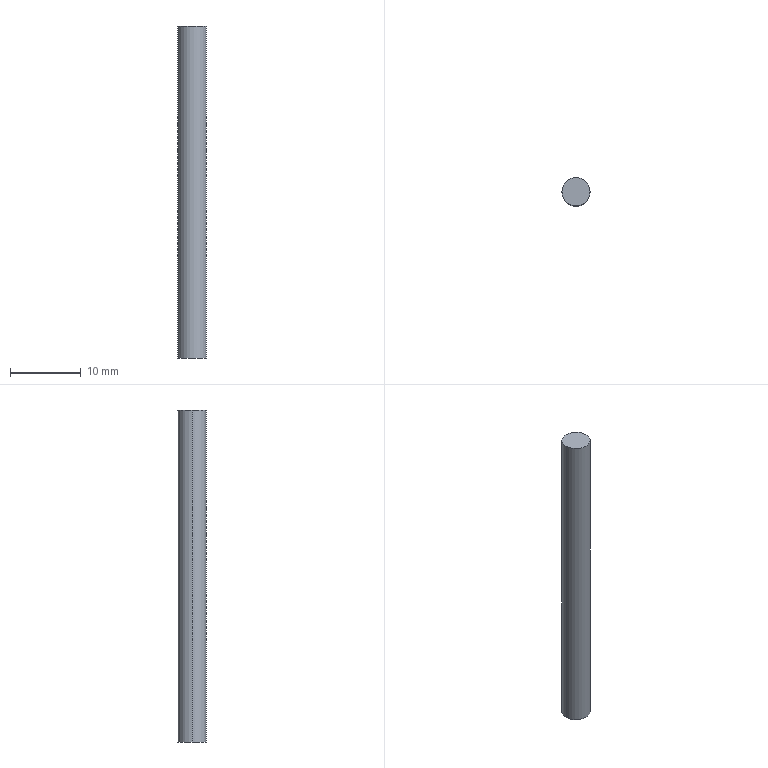Part | SolidWorks | features Extrusion 1 | 1 solid | 4 faces | box 4 x 4 x 47 mm | volume 590.619 mm3 | cylinder 2 | plane 2 | commonest cylinder face diameters 4 x2
STEP:
#1=CARTESIAN_POINT('',(2.,0.,47.));
#2=VERTEX_POINT('',#1);
#3=CARTESIAN_POINT('',(-2.,0.,47.));
#4=VERTEX_POINT('',#3);
#5=CARTESIAN_POINT('',(0.,0.,47.));
#6=DIRECTION('',(0.,0.,1.));
#7=DIRECTION('',(1.,0.,0.));
#8=AXIS2_PLACEMENT_3D('',#5,#6,#7);
#9=CIRCLE('',#8,2.);
#10=EDGE_CURVE('',#2,#4,#9,.T.);
#11=ORIENTED_EDGE('',*,*,#10,.F.);
#12=CARTESIAN_POINT('',(2.,0.,0.));
#13=VERTEX_POINT('',#12);
#14=CARTESIAN_POINT('',(2.,0.,47.));
#15=DIRECTION('',(0.,0.,-1.));
#16=VECTOR('',#15,1000.);
#17=LINE('',#14,#16);
#18=EDGE_CURVE('',#2,#13,#17,.T.);
#19=ORIENTED_EDGE('',*,*,#18,.T.);
#20=CARTESIAN_POINT('',(-2.,0.,0.));
#21=VERTEX_POINT('',#20);
#22=CARTESIAN_POINT('',(0.,0.,0.));
#23=DIRECTION('',(0.,0.,1.));
#24=DIRECTION('',(1.,0.,0.));
#25=AXIS2_PLACEMENT_3D('',#22,#23,#24);
#26=CIRCLE('',#25,2.);
#27=EDGE_CURVE('',#13,#21,#26,.T.);
#28=ORIENTED_EDGE('',*,*,#27,.T.);
#29=CARTESIAN_POINT('',(-2.,0.,47.));
#30=DIRECTION('',(0.,0.,-1.));
#31=VECTOR('',#30,1000.);
#32=LINE('',#29,#31);
#33=EDGE_CURVE('',#4,#21,#32,.T.);
#34=ORIENTED_EDGE('',*,*,#33,.F.);
#35=EDGE_LOOP('',(#11,#19,#28,#34));
#36=FACE_OUTER_BOUND('',#35,.T.);
#37=CARTESIAN_POINT('',(0.,0.,47.));
#38=DIRECTION('',(0.,0.,-1.));
#39=DIRECTION('',(-1.,0.,0.));
#40=AXIS2_PLACEMENT_3D('',#37,#38,#39);
#41=CYLINDRICAL_SURFACE('',#40,2.);
#42=ADVANCED_FACE('',(#36),#41,.T.);
#43=ORIENTED_EDGE('',*,*,#18,.F.);
#44=CARTESIAN_POINT('',(0.,0.,47.));
#45=DIRECTION('',(0.,0.,1.));
#46=DIRECTION('',(1.,0.,0.));
#47=AXIS2_PLACEMENT_3D('',#44,#45,#46);
#48=CIRCLE('',#47,2.);
#49=EDGE_CURVE('',#4,#2,#48,.T.);
#50=ORIENTED_EDGE('',*,*,#49,.F.);
#51=ORIENTED_EDGE('',*,*,#33,.T.);
#52=CARTESIAN_POINT('',(0.,0.,0.));
#53=DIRECTION('',(0.,0.,1.));
#54=DIRECTION('',(1.,0.,0.));
#55=AXIS2_PLACEMENT_3D('',#52,#53,#54);
#56=CIRCLE('',#55,2.);
#57=EDGE_CURVE('',#21,#13,#56,.T.);
#58=ORIENTED_EDGE('',*,*,#57,.T.);
#59=EDGE_LOOP('',(#43,#50,#51,#58));
#60=FACE_OUTER_BOUND('',#59,.T.);
#61=CARTESIAN_POINT('',(0.,0.,47.));
#62=DIRECTION('',(0.,0.,-1.));
#63=DIRECTION('',(-1.,0.,0.));
#64=AXIS2_PLACEMENT_3D('',#61,#62,#63);
#65=CYLINDRICAL_SURFACE('',#64,2.);
#66=ADVANCED_FACE('',(#60),#65,.T.);
#67=ORIENTED_EDGE('',*,*,#49,.T.);
#68=ORIENTED_EDGE('',*,*,#10,.T.);
#69=EDGE_LOOP('',(#67,#68));
#70=FACE_OUTER_BOUND('',#69,.T.);
#71=CARTESIAN_POINT('',(0.,0.,47.));
#72=DIRECTION('',(0.,0.,1.));
#73=DIRECTION('',(1.,0.,0.));
#74=AXIS2_PLACEMENT_3D('',#71,#72,#73);
#75=PLANE('',#74);
#76=ADVANCED_FACE('',(#70),#75,.T.);
#77=ORIENTED_EDGE('',*,*,#57,.F.);
#78=ORIENTED_EDGE('',*,*,#27,.F.);
#79=EDGE_LOOP('',(#77,#78));
#80=FACE_OUTER_BOUND('',#79,.T.);
#81=CARTESIAN_POINT('',(0.,0.,0.));
#82=DIRECTION('',(0.,0.,1.));
#83=DIRECTION('',(1.,0.,0.));
#84=AXIS2_PLACEMENT_3D('',#81,#82,#83);
#85=PLANE('',#84);
#86=ADVANCED_FACE('',(#80),#85,.F.);
#87=CLOSED_SHELL('',(#42,#66,#76,#86));
#88=MANIFOLD_SOLID_BREP('',#87);
#89=CARTESIAN_POINT('',(0.,0.,0.));
#90=DIRECTION('',(0.,0.,1.));
#91=DIRECTION('',(1.,0.,0.));
#92=AXIS2_PLACEMENT_3D('',#89,#90,#91);
#93=(LENGTH_UNIT()NAMED_UNIT(*)SI_UNIT(.MILLI.,.METRE.));
#94=UNCERTAINTY_MEASURE_WITH_UNIT(LENGTH_MEASURE(0.00001),#93,'','');
#95=(NAMED_UNIT(*)PLANE_ANGLE_UNIT()SI_UNIT($,.RADIAN.));
#96=(NAMED_UNIT(*)SI_UNIT($,.STERADIAN.)SOLID_ANGLE_UNIT());
#97=(GEOMETRIC_REPRESENTATION_CONTEXT(3)GLOBAL_UNCERTAINTY_ASSIGNED_CONTEXT((#94))GLOBAL_UNIT_ASSIGNED_CONTEXT((#93,#95,#96))REPRESENTATION_CONTEXT('',''));
#98=ADVANCED_BREP_SHAPE_REPRESENTATION('',(#88,#92),#97);